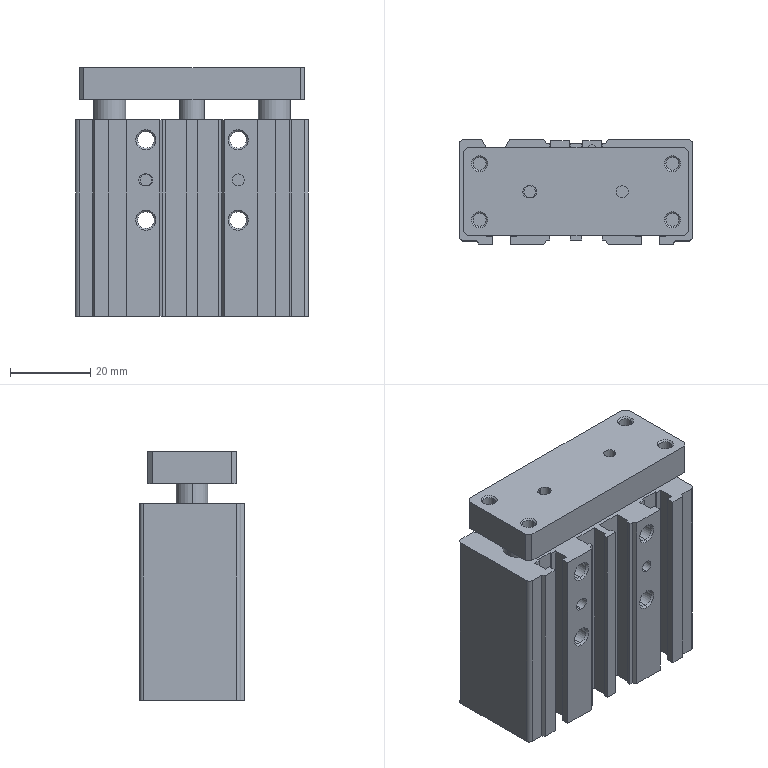Part | STEP file | Bag feed cylinder MGPM12-20-Z76L (0) | 1 solid | 266 faces | box 58 x 26 x 62 mm | volume 70641 mm3 | plane 136 | cylinder 82 | cone 48 | commonest cylinder face diameters 3 x16 3.24 x16 8 x12 4.019 x8 4.13 x8 4.3 x8